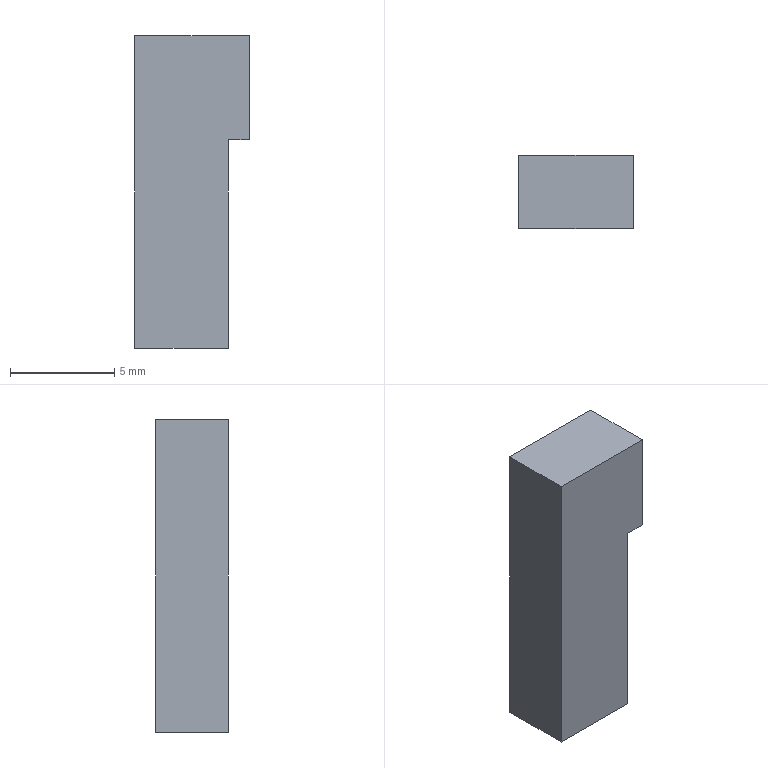Part | STEP file | gslz 2016.10.28-10_id1610_x_t | 1 solid | 8 faces | box 5.5 x 3.5 x 15 mm | volume 253.75 mm3 | plane 8
STEP:
#1=CARTESIAN_POINT('',(0.,0.,0.));
#2=DIRECTION('',(0.,0.,1.));
#3=DIRECTION('',(1.,0.,0.));
#4=AXIS2_PLACEMENT_3D('',#1,#2,#3);
#5=CARTESIAN_POINT('',(-688.56,84.249,15.));
#6=VERTEX_POINT('',#5);
#7=CARTESIAN_POINT('',(-694.06,84.249,15.));
#8=VERTEX_POINT('',#7);
#9=CARTESIAN_POINT('',(-691.31,84.249,15.));
#10=DIRECTION('',(-1.,0.000000055,0.));
#11=VECTOR('',#10,1.);
#12=LINE('',#9,#11);
#13=CARTESIAN_POINT('',(-694.06,84.249,15.));
#14=DIRECTION('',(-0.000000055,-1.,0.));
#15=DIRECTION('',(-1.,0.000000055,0.));
#16=AXIS2_PLACEMENT_3D('',#13,#14,#15);
#17=PLANE('',#16);
#18=CARTESIAN_POINT('',(-2.75,0.));
#19=DIRECTION('',(1.,0.));
#20=VECTOR('',#19,1.);
#21=LINE('',#18,#20);
#22=(GEOMETRIC_REPRESENTATION_CONTEXT(2)PARAMETRIC_REPRESENTATION_CONTEXT()REPRESENTATION_CONTEXT('',''));
#23=DEFINITIONAL_REPRESENTATION('',(#21),#22);
#24=PCURVE('',#17,#23);
#25=CARTESIAN_POINT('',(-694.06,85.999,15.));
#26=DIRECTION('',(0.,0.,1.));
#27=DIRECTION('',(1.,0.,0.));
#28=AXIS2_PLACEMENT_3D('',#25,#26,#27);
#29=PLANE('',#28);
#30=CARTESIAN_POINT('',(2.75,-1.75));
#31=DIRECTION('',(-1.,0.000000055));
#32=VECTOR('',#31,1.);
#33=LINE('',#30,#32);
#34=(GEOMETRIC_REPRESENTATION_CONTEXT(2)PARAMETRIC_REPRESENTATION_CONTEXT()REPRESENTATION_CONTEXT('',''));
#35=DEFINITIONAL_REPRESENTATION('',(#33),#34);
#36=PCURVE('',#29,#35);
#37=SURFACE_CURVE('',#12,(#24,#36),.PCURVE_S1.);
#38=EDGE_CURVE('',#6,#8,#37,.T.);
#39=ORIENTED_EDGE('',*,*,#38,.T.);
#40=CARTESIAN_POINT('',(-694.06,84.249,0.));
#41=VERTEX_POINT('',#40);
#42=CARTESIAN_POINT('',(-694.06,84.249,15.));
#43=DIRECTION('',(0.,0.,1.));
#44=VECTOR('',#43,1.);
#45=LINE('',#42,#44);
#46=CARTESIAN_POINT('',(0.,0.));
#47=DIRECTION('',(0.,-1.));
#48=VECTOR('',#47,1.);
#49=LINE('',#46,#48);
#50=(GEOMETRIC_REPRESENTATION_CONTEXT(2)PARAMETRIC_REPRESENTATION_CONTEXT()REPRESENTATION_CONTEXT('',''));
#51=DEFINITIONAL_REPRESENTATION('',(#49),#50);
#52=PCURVE('',#17,#51);
#53=CARTESIAN_POINT('',(-694.06,87.749,15.));
#54=DIRECTION('',(-1.,0.,0.));
#55=DIRECTION('',(0.,1.,0.));
#56=AXIS2_PLACEMENT_3D('',#53,#54,#55);
#57=PLANE('',#56);
#58=CARTESIAN_POINT('',(-3.5,0.));
#59=DIRECTION('',(0.,-1.));
#60=VECTOR('',#59,1.);
#61=LINE('',#58,#60);
#62=(GEOMETRIC_REPRESENTATION_CONTEXT(2)PARAMETRIC_REPRESENTATION_CONTEXT()REPRESENTATION_CONTEXT('',''));
#63=DEFINITIONAL_REPRESENTATION('',(#61),#62);
#64=PCURVE('',#57,#63);
#65=SURFACE_CURVE('',#45,(#52,#64),.PCURVE_S1.);
#66=EDGE_CURVE('',#41,#8,#65,.T.);
#67=ORIENTED_EDGE('',*,*,#66,.F.);
#68=CARTESIAN_POINT('',(-689.56,84.249,0.));
#69=VERTEX_POINT('',#68);
#70=CARTESIAN_POINT('',(-691.31,84.249,0.));
#71=DIRECTION('',(-1.,0.000000055,0.));
#72=VECTOR('',#71,1.);
#73=LINE('',#70,#72);
#74=CARTESIAN_POINT('',(-2.75,15.));
#75=DIRECTION('',(1.,0.));
#76=VECTOR('',#75,1.);
#77=LINE('',#74,#76);
#78=(GEOMETRIC_REPRESENTATION_CONTEXT(2)PARAMETRIC_REPRESENTATION_CONTEXT()REPRESENTATION_CONTEXT('',''));
#79=DEFINITIONAL_REPRESENTATION('',(#77),#78);
#80=PCURVE('',#17,#79);
#81=CARTESIAN_POINT('',(-694.06,85.999,0.));
#82=DIRECTION('',(0.,0.,1.));
#83=DIRECTION('',(1.,0.,0.));
#84=AXIS2_PLACEMENT_3D('',#81,#82,#83);
#85=PLANE('',#84);
#86=CARTESIAN_POINT('',(2.75,-1.75));
#87=DIRECTION('',(-1.,0.000000055));
#88=VECTOR('',#87,1.);
#89=LINE('',#86,#88);
#90=(GEOMETRIC_REPRESENTATION_CONTEXT(2)PARAMETRIC_REPRESENTATION_CONTEXT()REPRESENTATION_CONTEXT('',''));
#91=DEFINITIONAL_REPRESENTATION('',(#89),#90);
#92=PCURVE('',#85,#91);
#93=SURFACE_CURVE('',#73,(#80,#92),.PCURVE_S1.);
#94=EDGE_CURVE('',#69,#41,#93,.T.);
#95=ORIENTED_EDGE('',*,*,#94,.F.);
#96=CARTESIAN_POINT('',(-689.56,84.249,10.));
#97=VERTEX_POINT('',#96);
#98=CARTESIAN_POINT('',(-689.56,84.249,15.));
#99=DIRECTION('',(0.,0.,-1.));
#100=VECTOR('',#99,1.);
#101=LINE('',#98,#100);
#102=CARTESIAN_POINT('',(-4.5,0.));
#103=DIRECTION('',(0.,1.));
#104=VECTOR('',#103,1.);
#105=LINE('',#102,#104);
#106=(GEOMETRIC_REPRESENTATION_CONTEXT(2)PARAMETRIC_REPRESENTATION_CONTEXT()REPRESENTATION_CONTEXT('',''));
#107=DEFINITIONAL_REPRESENTATION('',(#105),#106);
#108=PCURVE('',#17,#107);
#109=CARTESIAN_POINT('',(-689.56,85.999,7.5));
#110=DIRECTION('',(1.,0.,0.));
#111=DIRECTION('',(0.,0.,-1.));
#112=AXIS2_PLACEMENT_3D('',#109,#110,#111);
#113=PLANE('',#112);
#114=CARTESIAN_POINT('',(-7.5,-1.75));
#115=DIRECTION('',(1.,0.));
#116=VECTOR('',#115,1.);
#117=LINE('',#114,#116);
#118=(GEOMETRIC_REPRESENTATION_CONTEXT(2)PARAMETRIC_REPRESENTATION_CONTEXT()REPRESENTATION_CONTEXT('',''));
#119=DEFINITIONAL_REPRESENTATION('',(#117),#118);
#120=PCURVE('',#113,#119);
#121=SURFACE_CURVE('',#101,(#108,#120),.PCURVE_S1.);
#122=EDGE_CURVE('',#97,#69,#121,.T.);
#123=ORIENTED_EDGE('',*,*,#122,.F.);
#124=CARTESIAN_POINT('',(-688.56,84.249,10.));
#125=VERTEX_POINT('',#124);
#126=CARTESIAN_POINT('',(-694.06,84.249,10.));
#127=DIRECTION('',(-1.,0.000000055,0.));
#128=VECTOR('',#127,1.);
#129=LINE('',#126,#128);
#130=CARTESIAN_POINT('',(0.,5.));
#131=DIRECTION('',(1.,0.));
#132=VECTOR('',#131,1.);
#133=LINE('',#130,#132);
#134=(GEOMETRIC_REPRESENTATION_CONTEXT(2)PARAMETRIC_REPRESENTATION_CONTEXT()REPRESENTATION_CONTEXT('',''));
#135=DEFINITIONAL_REPRESENTATION('',(#133),#134);
#136=PCURVE('',#17,#135);
#137=CARTESIAN_POINT('',(-694.06,85.999,10.));
#138=DIRECTION('',(0.,0.,1.));
#139=DIRECTION('',(1.,0.,0.));
#140=AXIS2_PLACEMENT_3D('',#137,#138,#139);
#141=PLANE('',#140);
#142=CARTESIAN_POINT('',(0.,-1.75));
#143=DIRECTION('',(-1.,0.000000055));
#144=VECTOR('',#143,1.);
#145=LINE('',#142,#144);
#146=(GEOMETRIC_REPRESENTATION_CONTEXT(2)PARAMETRIC_REPRESENTATION_CONTEXT()REPRESENTATION_CONTEXT('',''));
#147=DEFINITIONAL_REPRESENTATION('',(#145),#146);
#148=PCURVE('',#141,#147);
#149=SURFACE_CURVE('',#129,(#136,#148),.PCURVE_S1.);
#150=EDGE_CURVE('',#125,#97,#149,.T.);
#151=ORIENTED_EDGE('',*,*,#150,.F.);
#152=CARTESIAN_POINT('',(-688.56,84.249,15.));
#153=DIRECTION('',(0.,0.,1.));
#154=VECTOR('',#153,1.);
#155=LINE('',#152,#154);
#156=CARTESIAN_POINT('',(-5.5,0.));
#157=DIRECTION('',(0.,-1.));
#158=VECTOR('',#157,1.);
#159=LINE('',#156,#158);
#160=(GEOMETRIC_REPRESENTATION_CONTEXT(2)PARAMETRIC_REPRESENTATION_CONTEXT()REPRESENTATION_CONTEXT('',''));
#161=DEFINITIONAL_REPRESENTATION('',(#159),#160);
#162=PCURVE('',#17,#161);
#163=CARTESIAN_POINT('',(-688.56,84.249,15.));
#164=DIRECTION('',(1.,0.,0.));
#165=DIRECTION('',(0.,-1.,0.));
#166=AXIS2_PLACEMENT_3D('',#163,#164,#165);
#167=PLANE('',#166);
#168=CARTESIAN_POINT('',(0.,0.));
#169=DIRECTION('',(0.,-1.));
#170=VECTOR('',#169,1.);
#171=LINE('',#168,#170);
#172=(GEOMETRIC_REPRESENTATION_CONTEXT(2)PARAMETRIC_REPRESENTATION_CONTEXT()REPRESENTATION_CONTEXT('',''));
#173=DEFINITIONAL_REPRESENTATION('',(#171),#172);
#174=PCURVE('',#167,#173);
#175=SURFACE_CURVE('',#155,(#162,#174),.PCURVE_S1.);
#176=EDGE_CURVE('',#125,#6,#175,.T.);
#177=ORIENTED_EDGE('',*,*,#176,.T.);
#178=EDGE_LOOP('',(#39,#67,#95,#123,#151,#177));
#179=FACE_BOUND('',#178,.T.);
#180=ADVANCED_FACE('',(#179),#17,.T.);
#181=CARTESIAN_POINT('',(-694.06,87.749,0.));
#182=VERTEX_POINT('',#181);
#183=CARTESIAN_POINT('',(-689.56,87.749,0.));
#184=VERTEX_POINT('',#183);
#185=CARTESIAN_POINT('',(-691.31,87.749,0.));
#186=DIRECTION('',(1.,-0.000000055,0.));
#187=VECTOR('',#186,1.);
#188=LINE('',#185,#187);
#189=CARTESIAN_POINT('',(-688.56,87.749,15.));
#190=DIRECTION('',(0.000000055,1.,0.));
#191=DIRECTION('',(1.,-0.000000055,0.));
#192=AXIS2_PLACEMENT_3D('',#189,#190,#191);
#193=PLANE('',#192);
#194=CARTESIAN_POINT('',(-2.75,15.));
#195=DIRECTION('',(1.,0.));
#196=VECTOR('',#195,1.);
#197=LINE('',#194,#196);
#198=(GEOMETRIC_REPRESENTATION_CONTEXT(2)PARAMETRIC_REPRESENTATION_CONTEXT()REPRESENTATION_CONTEXT('',''));
#199=DEFINITIONAL_REPRESENTATION('',(#197),#198);
#200=PCURVE('',#193,#199);
#201=CARTESIAN_POINT('',(2.75,1.75));
#202=DIRECTION('',(1.,-0.000000055));
#203=VECTOR('',#202,1.);
#204=LINE('',#201,#203);
#205=(GEOMETRIC_REPRESENTATION_CONTEXT(2)PARAMETRIC_REPRESENTATION_CONTEXT()REPRESENTATION_CONTEXT('',''));
#206=DEFINITIONAL_REPRESENTATION('',(#204),#205);
#207=PCURVE('',#85,#206);
#208=SURFACE_CURVE('',#188,(#200,#207),.PCURVE_S1.);
#209=EDGE_CURVE('',#182,#184,#208,.T.);
#210=ORIENTED_EDGE('',*,*,#209,.F.);
#211=CARTESIAN_POINT('',(-694.06,87.749,15.));
#212=VERTEX_POINT('',#211);
#213=CARTESIAN_POINT('',(-694.06,87.749,15.));
#214=DIRECTION('',(0.,0.,1.));
#215=VECTOR('',#214,1.);
#216=LINE('',#213,#215);
#217=CARTESIAN_POINT('',(-5.5,0.));
#218=DIRECTION('',(0.,-1.));
#219=VECTOR('',#218,1.);
#220=LINE('',#217,#219);
#221=(GEOMETRIC_REPRESENTATION_CONTEXT(2)PARAMETRIC_REPRESENTATION_CONTEXT()REPRESENTATION_CONTEXT('',''));
#222=DEFINITIONAL_REPRESENTATION('',(#220),#221);
#223=PCURVE('',#193,#222);
#224=CARTESIAN_POINT('',(0.,0.));
#225=DIRECTION('',(0.,-1.));
#226=VECTOR('',#225,1.);
#227=LINE('',#224,#226);
#228=(GEOMETRIC_REPRESENTATION_CONTEXT(2)PARAMETRIC_REPRESENTATION_CONTEXT()REPRESENTATION_CONTEXT('',''));
#229=DEFINITIONAL_REPRESENTATION('',(#227),#228);
#230=PCURVE('',#57,#229);
#231=SURFACE_CURVE('',#216,(#223,#230),.PCURVE_S1.);
#232=EDGE_CURVE('',#182,#212,#231,.T.);
#233=ORIENTED_EDGE('',*,*,#232,.T.);
#234=CARTESIAN_POINT('',(-688.56,87.749,15.));
#235=VERTEX_POINT('',#234);
#236=CARTESIAN_POINT('',(-691.31,87.749,15.));
#237=DIRECTION('',(1.,-0.000000055,0.));
#238=VECTOR('',#237,1.);
#239=LINE('',#236,#238);
#240=CARTESIAN_POINT('',(-2.75,0.));
#241=DIRECTION('',(1.,0.));
#242=VECTOR('',#241,1.);
#243=LINE('',#240,#242);
#244=(GEOMETRIC_REPRESENTATION_CONTEXT(2)PARAMETRIC_REPRESENTATION_CONTEXT()REPRESENTATION_CONTEXT('',''));
#245=DEFINITIONAL_REPRESENTATION('',(#243),#244);
#246=PCURVE('',#193,#245);
#247=CARTESIAN_POINT('',(2.75,1.75));
#248=DIRECTION('',(1.,-0.000000055));
#249=VECTOR('',#248,1.);
#250=LINE('',#247,#249);
#251=(GEOMETRIC_REPRESENTATION_CONTEXT(2)PARAMETRIC_REPRESENTATION_CONTEXT()REPRESENTATION_CONTEXT('',''));
#252=DEFINITIONAL_REPRESENTATION('',(#250),#251);
#253=PCURVE('',#29,#252);
#254=SURFACE_CURVE('',#239,(#246,#253),.PCURVE_S1.);
#255=EDGE_CURVE('',#212,#235,#254,.T.);
#256=ORIENTED_EDGE('',*,*,#255,.T.);
#257=CARTESIAN_POINT('',(-688.56,87.749,10.));
#258=VERTEX_POINT('',#257);
#259=CARTESIAN_POINT('',(-688.56,87.749,15.));
#260=DIRECTION('',(0.,0.,1.));
#261=VECTOR('',#260,1.);
#262=LINE('',#259,#261);
#263=CARTESIAN_POINT('',(0.,0.));
#264=DIRECTION('',(0.,-1.));
#265=VECTOR('',#264,1.);
#266=LINE('',#263,#265);
#267=(GEOMETRIC_REPRESENTATION_CONTEXT(2)PARAMETRIC_REPRESENTATION_CONTEXT()REPRESENTATION_CONTEXT('',''));
#268=DEFINITIONAL_REPRESENTATION('',(#266),#267);
#269=PCURVE('',#193,#268);
#270=CARTESIAN_POINT('',(-3.5,0.));
#271=DIRECTION('',(0.,-1.));
#272=VECTOR('',#271,1.);
#273=LINE('',#270,#272);
#274=(GEOMETRIC_REPRESENTATION_CONTEXT(2)PARAMETRIC_REPRESENTATION_CONTEXT()REPRESENTATION_CONTEXT('',''));
#275=DEFINITIONAL_REPRESENTATION('',(#273),#274);
#276=PCURVE('',#167,#275);
#277=SURFACE_CURVE('',#262,(#269,#276),.PCURVE_S1.);
#278=EDGE_CURVE('',#258,#235,#277,.T.);
#279=ORIENTED_EDGE('',*,*,#278,.F.);
#280=CARTESIAN_POINT('',(-689.56,87.749,10.));
#281=VERTEX_POINT('',#280);
#282=CARTESIAN_POINT('',(-688.56,87.749,10.));
#283=DIRECTION('',(1.,-0.000000055,0.));
#284=VECTOR('',#283,1.);
#285=LINE('',#282,#284);
#286=CARTESIAN_POINT('',(0.,5.));
#287=DIRECTION('',(1.,0.));
#288=VECTOR('',#287,1.);
#289=LINE('',#286,#288);
#290=(GEOMETRIC_REPRESENTATION_CONTEXT(2)PARAMETRIC_REPRESENTATION_CONTEXT()REPRESENTATION_CONTEXT('',''));
#291=DEFINITIONAL_REPRESENTATION('',(#289),#290);
#292=PCURVE('',#193,#291);
#293=CARTESIAN_POINT('',(5.5,1.75));
#294=DIRECTION('',(1.,-0.000000055));
#295=VECTOR('',#294,1.);
#296=LINE('',#293,#295);
#297=(GEOMETRIC_REPRESENTATION_CONTEXT(2)PARAMETRIC_REPRESENTATION_CONTEXT()REPRESENTATION_CONTEXT('',''));
#298=DEFINITIONAL_REPRESENTATION('',(#296),#297);
#299=PCURVE('',#141,#298);
#300=SURFACE_CURVE('',#285,(#292,#299),.PCURVE_S1.);
#301=EDGE_CURVE('',#281,#258,#300,.T.);
#302=ORIENTED_EDGE('',*,*,#301,.F.);
#303=CARTESIAN_POINT('',(-689.56,87.749,15.));
#304=DIRECTION('',(0.,0.,1.));
#305=VECTOR('',#304,1.);
#306=LINE('',#303,#305);
#307=CARTESIAN_POINT('',(-1.,0.));
#308=DIRECTION('',(0.,-1.));
#309=VECTOR('',#308,1.);
#310=LINE('',#307,#309);
#311=(GEOMETRIC_REPRESENTATION_CONTEXT(2)PARAMETRIC_REPRESENTATION_CONTEXT()REPRESENTATION_CONTEXT('',''));
#312=DEFINITIONAL_REPRESENTATION('',(#310),#311);
#313=PCURVE('',#193,#312);
#314=CARTESIAN_POINT('',(-7.5,1.75));
#315=DIRECTION('',(-1.,0.));
#316=VECTOR('',#315,1.);
#317=LINE('',#314,#316);
#318=(GEOMETRIC_REPRESENTATION_CONTEXT(2)PARAMETRIC_REPRESENTATION_CONTEXT()REPRESENTATION_CONTEXT('',''));
#319=DEFINITIONAL_REPRESENTATION('',(#317),#318);
#320=PCURVE('',#113,#319);
#321=SURFACE_CURVE('',#306,(#313,#320),.PCURVE_S1.);
#322=EDGE_CURVE('',#184,#281,#321,.T.);
#323=ORIENTED_EDGE('',*,*,#322,.F.);
#324=EDGE_LOOP('',(#210,#233,#256,#279,#302,#323));
#325=FACE_BOUND('',#324,.T.);
#326=ADVANCED_FACE('',(#325),#193,.T.);
#327=ORIENTED_EDGE('',*,*,#255,.F.);
#328=CARTESIAN_POINT('',(-694.06,85.999,15.));
#329=DIRECTION('',(0.,1.,0.));
#330=VECTOR('',#329,1.);
#331=LINE('',#328,#330);
#332=CARTESIAN_POINT('',(0.,0.));
#333=DIRECTION('',(0.,1.));
#334=VECTOR('',#333,1.);
#335=LINE('',#332,#334);
#336=(GEOMETRIC_REPRESENTATION_CONTEXT(2)PARAMETRIC_REPRESENTATION_CONTEXT()REPRESENTATION_CONTEXT('',''));
#337=DEFINITIONAL_REPRESENTATION('',(#335),#336);
#338=PCURVE('',#29,#337);
#339=CARTESIAN_POINT('',(-1.75,0.));
#340=DIRECTION('',(1.,0.));
#341=VECTOR('',#340,1.);
#342=LINE('',#339,#341);
#343=(GEOMETRIC_REPRESENTATION_CONTEXT(2)PARAMETRIC_REPRESENTATION_CONTEXT()REPRESENTATION_CONTEXT('',''));
#344=DEFINITIONAL_REPRESENTATION('',(#342),#343);
#345=PCURVE('',#57,#344);
#346=SURFACE_CURVE('',#331,(#338,#345),.PCURVE_S1.);
#347=EDGE_CURVE('',#8,#212,#346,.T.);
#348=ORIENTED_EDGE('',*,*,#347,.F.);
#349=ORIENTED_EDGE('',*,*,#38,.F.);
#350=CARTESIAN_POINT('',(-688.56,85.999,15.));
#351=DIRECTION('',(0.,-1.,0.));
#352=VECTOR('',#351,1.);
#353=LINE('',#350,#352);
#354=CARTESIAN_POINT('',(5.5,-0.000000303));
#355=DIRECTION('',(0.,-1.));
#356=VECTOR('',#355,1.);
#357=LINE('',#354,#356);
#358=(GEOMETRIC_REPRESENTATION_CONTEXT(2)PARAMETRIC_REPRESENTATION_CONTEXT()REPRESENTATION_CONTEXT('',''));
#359=DEFINITIONAL_REPRESENTATION('',(#357),#358);
#360=PCURVE('',#29,#359);
#361=CARTESIAN_POINT('',(-1.75,0.));
#362=DIRECTION('',(1.,0.));
#363=VECTOR('',#362,1.);
#364=LINE('',#361,#363);
#365=(GEOMETRIC_REPRESENTATION_CONTEXT(2)PARAMETRIC_REPRESENTATION_CONTEXT()REPRESENTATION_CONTEXT('',''));
#366=DEFINITIONAL_REPRESENTATION('',(#364),#365);
#367=PCURVE('',#167,#366);
#368=SURFACE_CURVE('',#353,(#360,#367),.PCURVE_S1.);
#369=EDGE_CURVE('',#235,#6,#368,.T.);
#370=ORIENTED_EDGE('',*,*,#369,.F.);
#371=EDGE_LOOP('',(#327,#348,#349,#370));
#372=FACE_BOUND('',#371,.T.);
#373=ADVANCED_FACE('',(#372),#29,.T.);
#374=CARTESIAN_POINT('',(-689.56,85.999,0.));
#375=DIRECTION('',(0.,-1.,0.));
#376=VECTOR('',#375,1.);
#377=LINE('',#374,#376);
#378=CARTESIAN_POINT('',(4.5,0.));
#379=DIRECTION('',(0.,-1.));
#380=VECTOR('',#379,1.);
#381=LINE('',#378,#380);
#382=(GEOMETRIC_REPRESENTATION_CONTEXT(2)PARAMETRIC_REPRESENTATION_CONTEXT()REPRESENTATION_CONTEXT('',''));
#383=DEFINITIONAL_REPRESENTATION('',(#381),#382);
#384=PCURVE('',#85,#383);
#385=CARTESIAN_POINT('',(7.5,0.000000303));
#386=DIRECTION('',(0.,-1.));
#387=VECTOR('',#386,1.);
#388=LINE('',#385,#387);
#389=(GEOMETRIC_REPRESENTATION_CONTEXT(2)PARAMETRIC_REPRESENTATION_CONTEXT()REPRESENTATION_CONTEXT('',''));
#390=DEFINITIONAL_REPRESENTATION('',(#388),#389);
#391=PCURVE('',#113,#390);
#392=SURFACE_CURVE('',#377,(#384,#391),.PCURVE_S1.);
#393=EDGE_CURVE('',#184,#69,#392,.T.);
#394=ORIENTED_EDGE('',*,*,#393,.T.);
#395=ORIENTED_EDGE('',*,*,#94,.T.);
#396=CARTESIAN_POINT('',(-694.06,85.999,0.));
#397=DIRECTION('',(0.,1.,0.));
#398=VECTOR('',#397,1.);
#399=LINE('',#396,#398);
#400=CARTESIAN_POINT('',(0.,0.));
#401=DIRECTION('',(0.,1.));
#402=VECTOR('',#401,1.);
#403=LINE('',#400,#402);
#404=(GEOMETRIC_REPRESENTATION_CONTEXT(2)PARAMETRIC_REPRESENTATION_CONTEXT()REPRESENTATION_CONTEXT('',''));
#405=DEFINITIONAL_REPRESENTATION('',(#403),#404);
#406=PCURVE('',#85,#405);
#407=CARTESIAN_POINT('',(-1.75,15.));
#408=DIRECTION('',(1.,0.));
#409=VECTOR('',#408,1.);
#410=LINE('',#407,#409);
#411=(GEOMETRIC_REPRESENTATION_CONTEXT(2)PARAMETRIC_REPRESENTATION_CONTEXT()REPRESENTATION_CONTEXT('',''));
#412=DEFINITIONAL_REPRESENTATION('',(#410),#411);
#413=PCURVE('',#57,#412);
#414=SURFACE_CURVE('',#399,(#406,#413),.PCURVE_S1.);
#415=EDGE_CURVE('',#41,#182,#414,.T.);
#416=ORIENTED_EDGE('',*,*,#415,.T.);
#417=ORIENTED_EDGE('',*,*,#209,.T.);
#418=EDGE_LOOP('',(#394,#395,#416,#417));
#419=FACE_BOUND('',#418,.T.);
#420=ADVANCED_FACE('',(#419),#85,.F.);
#421=ORIENTED_EDGE('',*,*,#415,.F.);
#422=ORIENTED_EDGE('',*,*,#66,.T.);
#423=ORIENTED_EDGE('',*,*,#347,.T.);
#424=ORIENTED_EDGE('',*,*,#232,.F.);
#425=EDGE_LOOP('',(#421,#422,#423,#424));
#426=FACE_BOUND('',#425,.T.);
#427=ADVANCED_FACE('',(#426),#57,.T.);
#428=CARTESIAN_POINT('',(-689.56,85.999,10.));
#429=DIRECTION('',(0.,1.,0.));
#430=VECTOR('',#429,1.);
#431=LINE('',#428,#430);
#432=CARTESIAN_POINT('',(-2.5,0.000000303));
#433=DIRECTION('',(0.,1.));
#434=VECTOR('',#433,1.);
#435=LINE('',#432,#434);
#436=(GEOMETRIC_REPRESENTATION_CONTEXT(2)PARAMETRIC_REPRESENTATION_CONTEXT()REPRESENTATION_CONTEXT('',''));
#437=DEFINITIONAL_REPRESENTATION('',(#435),#436);
#438=PCURVE('',#113,#437);
#439=CARTESIAN_POINT('',(4.5,0.));
#440=DIRECTION('',(0.,1.));
#441=VECTOR('',#440,1.);
#442=LINE('',#439,#441);
#443=(GEOMETRIC_REPRESENTATION_CONTEXT(2)PARAMETRIC_REPRESENTATION_CONTEXT()REPRESENTATION_CONTEXT('',''));
#444=DEFINITIONAL_REPRESENTATION('',(#442),#443);
#445=PCURVE('',#141,#444);
#446=SURFACE_CURVE('',#431,(#438,#445),.PCURVE_S1.);
#447=EDGE_CURVE('',#97,#281,#446,.T.);
#448=ORIENTED_EDGE('',*,*,#447,.F.);
#449=ORIENTED_EDGE('',*,*,#122,.T.);
#450=ORIENTED_EDGE('',*,*,#393,.F.);
#451=ORIENTED_EDGE('',*,*,#322,.T.);
#452=EDGE_LOOP('',(#448,#449,#450,#451));
#453=FACE_BOUND('',#452,.T.);
#454=ADVANCED_FACE('',(#453),#113,.T.);
#455=CARTESIAN_POINT('',(-688.56,84.249,10.));
#456=DIRECTION('',(0.,-1.,0.));
#457=VECTOR('',#456,1.);
#458=LINE('',#455,#457);
#459=CARTESIAN_POINT('',(0.,5.));
#460=DIRECTION('',(1.,0.));
#461=VECTOR('',#460,1.);
#462=LINE('',#459,#461);
#463=(GEOMETRIC_REPRESENTATION_CONTEXT(2)PARAMETRIC_REPRESENTATION_CONTEXT()REPRESENTATION_CONTEXT('',''));
#464=DEFINITIONAL_REPRESENTATION('',(#462),#463);
#465=PCURVE('',#167,#464);
#466=CARTESIAN_POINT('',(5.5,-1.75));
#467=DIRECTION('',(0.,-1.));
#468=VECTOR('',#467,1.);
#469=LINE('',#466,#468);
#470=(GEOMETRIC_REPRESENTATION_CONTEXT(2)PARAMETRIC_REPRESENTATION_CONTEXT()REPRESENTATION_CONTEXT('',''));
#471=DEFINITIONAL_REPRESENTATION('',(#469),#470);
#472=PCURVE('',#141,#471);
#473=SURFACE_CURVE('',#458,(#465,#472),.PCURVE_S1.);
#474=EDGE_CURVE('',#258,#125,#473,.T.);
#475=ORIENTED_EDGE('',*,*,#474,.F.);
#476=ORIENTED_EDGE('',*,*,#278,.T.);
#477=ORIENTED_EDGE('',*,*,#369,.T.);
#478=ORIENTED_EDGE('',*,*,#176,.F.);
#479=EDGE_LOOP('',(#475,#476,#477,#478));
#480=FACE_BOUND('',#479,.T.);
#481=ADVANCED_FACE('',(#480),#167,.T.);
#482=ORIENTED_EDGE('',*,*,#301,.T.);
#483=ORIENTED_EDGE('',*,*,#474,.T.);
#484=ORIENTED_EDGE('',*,*,#150,.T.);
#485=ORIENTED_EDGE('',*,*,#447,.T.);
#486=EDGE_LOOP('',(#482,#483,#484,#485));
#487=FACE_BOUND('',#486,.T.);
#488=ADVANCED_FACE('',(#487),#141,.F.);
#489=CLOSED_SHELL('',(#180,#326,#373,#420,#427,#454,#481,#488));
#490=MANIFOLD_SOLID_BREP('',#489);
#491=(LENGTH_UNIT()NAMED_UNIT(*)SI_UNIT(.MILLI.,.METRE.));
#492=UNCERTAINTY_MEASURE_WITH_UNIT(LENGTH_MEASURE(0.0000001),#491,'','');
#493=(NAMED_UNIT(*)PLANE_ANGLE_UNIT()SI_UNIT($,.RADIAN.));
#494=(NAMED_UNIT(*)SI_UNIT($,.STERADIAN.)SOLID_ANGLE_UNIT());
#495=(GEOMETRIC_REPRESENTATION_CONTEXT(3)GLOBAL_UNCERTAINTY_ASSIGNED_CONTEXT((#492))GLOBAL_UNIT_ASSIGNED_CONTEXT((#491,#493,#494))REPRESENTATION_CONTEXT('',''));
#496=ADVANCED_BREP_SHAPE_REPRESENTATION('',(#4,#490),#495);